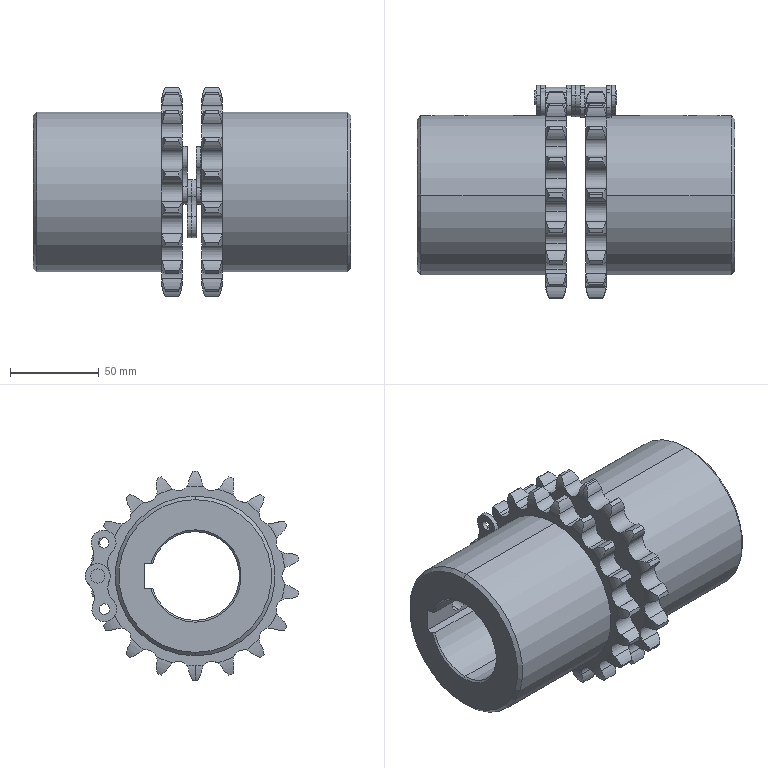Part | SolidWorks | features CompositeCurve 3 | 13 solids | 392 faces | box 178.9 x 120.134 x 117.94 mm | volume 791458 mm3 | cylinder 266 | torus 76 | plane 34 | cone 16 | commonest cylinder face diameters 28 x80 11.91 x56 117.94 x38 6 x36 14 x24 20 x16